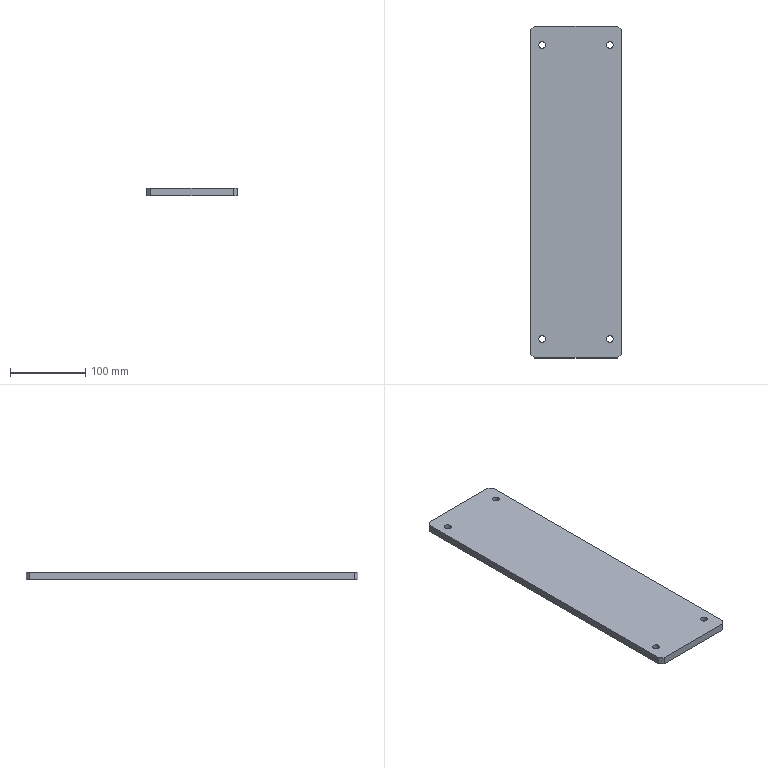Part | STEP file | POST.PLATE.1.stp | 1 solid | 18 faces | box 120 x 440 x 10 mm | volume 524955 mm3 | plane 10 | cylinder 4 | spline 4 | commonest cylinder face diameters 9 x4